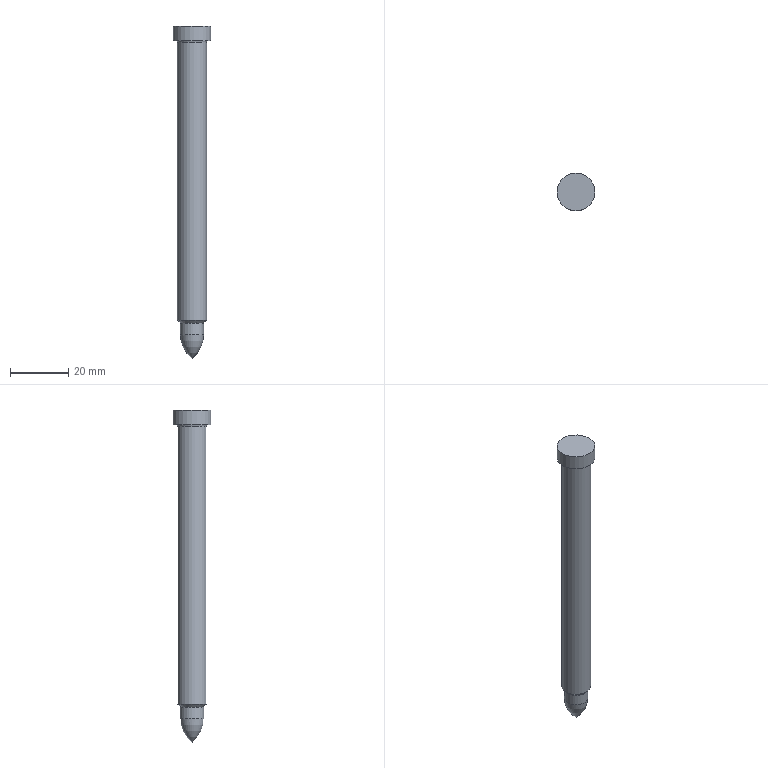Part | NX | features 8 2 | 1 solid | 9 faces | box 13 x 13 x 113.8 mm | volume 8684 mm3 | cylinder 3 | torus 3 | plane 2 | cone 1 | commonest cylinder face diameters 8 x1 10 x1 13 x1
STEP:
#1=CARTESIAN_POINT('',(3285.247,77.328,85.5));
#2=VERTEX_POINT('',#1);
#3=CARTESIAN_POINT('',(3290.247,77.328,85.5));
#4=DIRECTION('',(0.,0.,-1.));
#5=DIRECTION('',(1.,0.,0.));
#6=AXIS2_PLACEMENT_3D('',#3,#4,#5);
#7=CIRCLE('',#6,5.);
#8=EDGE_CURVE('',#2,#2,#7,.T.);
#9=ORIENTED_EDGE('',*,*,#8,.T.);
#10=EDGE_LOOP('',(#9));
#11=FACE_BOUND('',#10,.T.);
#12=CARTESIAN_POINT('',(3285.247,77.328,-9.8));
#13=VERTEX_POINT('',#12);
#14=CARTESIAN_POINT('',(3290.247,77.328,-9.8));
#15=DIRECTION('',(0.,0.,1.));
#16=DIRECTION('',(-1.,0.,0.));
#17=AXIS2_PLACEMENT_3D('',#14,#15,#16);
#18=CIRCLE('',#17,5.);
#19=EDGE_CURVE('',#13,#13,#18,.T.);
#20=ORIENTED_EDGE('',*,*,#19,.T.);
#21=EDGE_LOOP('',(#20));
#22=FACE_BOUND('',#21,.T.);
#23=CARTESIAN_POINT('',(3290.247,77.328,31.));
#24=DIRECTION('',(0.,0.,-1.));
#25=DIRECTION('',(-1.,0.,0.));
#26=AXIS2_PLACEMENT_3D('',#23,#24,#25);
#27=CYLINDRICAL_SURFACE('',#26,5.);
#28=ADVANCED_FACE('',(#11,#22),#27,.T.);
#29=CARTESIAN_POINT('',(3290.247,77.328,-22.8));
#30=VERTEX_POINT('',#29);
#31=VERTEX_LOOP('',#30);
#32=FACE_BOUND('',#31,.T.);
#33=CARTESIAN_POINT('',(3286.247,77.328,-14.8));
#34=VERTEX_POINT('',#33);
#35=CARTESIAN_POINT('',(3290.247,77.328,-14.8));
#36=DIRECTION('',(0.,0.,1.));
#37=DIRECTION('',(-1.,0.,0.));
#38=AXIS2_PLACEMENT_3D('',#35,#36,#37);
#39=CIRCLE('',#38,4.);
#40=EDGE_CURVE('',#34,#34,#39,.T.);
#41=ORIENTED_EDGE('',*,*,#40,.F.);
#42=EDGE_LOOP('',(#41));
#43=FACE_BOUND('',#42,.T.);
#44=CARTESIAN_POINT('',(3290.247,77.328,-14.8));
#45=DIRECTION('',(0.,0.,-1.));
#46=DIRECTION('',(-1.,0.,0.));
#47=AXIS2_PLACEMENT_3D('',#44,#45,#46);
#48=DEGENERATE_TOROIDAL_SURFACE('',#47,6.,10.,.F.);
#49=ADVANCED_FACE('',(#32,#43),#48,.F.);
#50=CARTESIAN_POINT('',(3286.159,77.328,-10.712));
#51=VERTEX_POINT('',#50);
#52=CARTESIAN_POINT('',(3290.247,77.328,-10.712));
#53=DIRECTION('',(0.,0.,1.));
#54=DIRECTION('',(1.,0.,0.));
#55=AXIS2_PLACEMENT_3D('',#52,#53,#54);
#56=CIRCLE('',#55,4.088);
#57=EDGE_CURVE('',#51,#51,#56,.T.);
#58=ORIENTED_EDGE('',*,*,#57,.F.);
#59=EDGE_LOOP('',(#58));
#60=FACE_BOUND('',#59,.T.);
#61=CARTESIAN_POINT('',(3286.247,77.328,-10.924));
#62=VERTEX_POINT('',#61);
#63=CARTESIAN_POINT('',(3290.247,77.328,-10.924));
#64=DIRECTION('',(0.,0.,-1.));
#65=DIRECTION('',(1.,0.,0.));
#66=AXIS2_PLACEMENT_3D('',#63,#64,#65);
#67=CIRCLE('',#66,4.);
#68=EDGE_CURVE('',#62,#62,#67,.T.);
#69=ORIENTED_EDGE('',*,*,#68,.F.);
#70=EDGE_LOOP('',(#69));
#71=FACE_BOUND('',#70,.T.);
#72=CARTESIAN_POINT('',(3290.247,77.328,-10.924));
#73=DIRECTION('',(0.,0.,-1.));
#74=DIRECTION('',(1.,0.,0.));
#75=AXIS2_PLACEMENT_3D('',#72,#73,#74);
#76=TOROIDAL_SURFACE('',#75,4.3,0.3);
#77=ADVANCED_FACE('',(#60,#71),#76,.F.);
#78=ORIENTED_EDGE('',*,*,#40,.T.);
#79=EDGE_LOOP('',(#78));
#80=FACE_BOUND('',#79,.T.);
#81=ORIENTED_EDGE('',*,*,#68,.T.);
#82=EDGE_LOOP('',(#81));
#83=FACE_BOUND('',#82,.T.);
#84=CARTESIAN_POINT('',(3290.247,77.328,-12.8));
#85=DIRECTION('',(0.,0.,-1.));
#86=DIRECTION('',(-1.,0.,0.));
#87=AXIS2_PLACEMENT_3D('',#84,#85,#86);
#88=CYLINDRICAL_SURFACE('',#87,4.);
#89=ADVANCED_FACE('',(#80,#83),#88,.T.);
#90=ORIENTED_EDGE('',*,*,#19,.F.);
#91=EDGE_LOOP('',(#90));
#92=FACE_BOUND('',#91,.T.);
#93=ORIENTED_EDGE('',*,*,#57,.T.);
#94=EDGE_LOOP('',(#93));
#95=FACE_BOUND('',#94,.T.);
#96=CARTESIAN_POINT('',(3290.247,77.328,-10.3));
#97=DIRECTION('',(0.,0.,1.));
#98=DIRECTION('',(-1.,0.,0.));
#99=AXIS2_PLACEMENT_3D('',#96,#97,#98);
#100=CONICAL_SURFACE('',#99,4.5,0.7854);
#101=ADVANCED_FACE('',(#92,#95),#100,.T.);
#102=ORIENTED_EDGE('',*,*,#8,.F.);
#103=EDGE_LOOP('',(#102));
#104=FACE_BOUND('',#103,.T.);
#105=CARTESIAN_POINT('',(3284.747,77.328,86.));
#106=VERTEX_POINT('',#105);
#107=CARTESIAN_POINT('',(3290.247,77.328,86.));
#108=DIRECTION('',(0.,0.,1.));
#109=DIRECTION('',(1.,0.,0.));
#110=AXIS2_PLACEMENT_3D('',#107,#108,#109);
#111=CIRCLE('',#110,5.5);
#112=EDGE_CURVE('',#106,#106,#111,.T.);
#113=ORIENTED_EDGE('',*,*,#112,.F.);
#114=EDGE_LOOP('',(#113));
#115=FACE_BOUND('',#114,.T.);
#116=CARTESIAN_POINT('',(3290.247,77.328,85.5));
#117=DIRECTION('',(0.,0.,1.));
#118=DIRECTION('',(1.,0.,0.));
#119=AXIS2_PLACEMENT_3D('',#116,#117,#118);
#120=TOROIDAL_SURFACE('',#119,5.5,0.5);
#121=ADVANCED_FACE('',(#104,#115),#120,.F.);
#122=CARTESIAN_POINT('',(3283.747,77.328,86.));
#123=VERTEX_POINT('',#122);
#124=CARTESIAN_POINT('',(3290.247,77.328,86.));
#125=DIRECTION('',(0.,0.,1.));
#126=DIRECTION('',(-1.,0.,0.));
#127=AXIS2_PLACEMENT_3D('',#124,#125,#126);
#128=CIRCLE('',#127,6.5);
#129=EDGE_CURVE('',#123,#123,#128,.T.);
#130=ORIENTED_EDGE('',*,*,#129,.F.);
#131=EDGE_LOOP('',(#130));
#132=FACE_BOUND('',#131,.T.);
#133=ORIENTED_EDGE('',*,*,#112,.T.);
#134=EDGE_LOOP('',(#133));
#135=FACE_BOUND('',#134,.T.);
#136=CARTESIAN_POINT('',(3290.247,77.328,86.));
#137=DIRECTION('',(0.,0.,-1.));
#138=DIRECTION('',(-1.,0.,0.));
#139=AXIS2_PLACEMENT_3D('',#136,#137,#138);
#140=PLANE('',#139);
#141=ADVANCED_FACE('',(#132,#135),#140,.T.);
#142=CARTESIAN_POINT('',(3283.747,77.328,91.));
#143=VERTEX_POINT('',#142);
#144=CARTESIAN_POINT('',(3290.247,77.328,91.));
#145=DIRECTION('',(0.,0.,-1.));
#146=DIRECTION('',(-1.,0.,0.));
#147=AXIS2_PLACEMENT_3D('',#144,#145,#146);
#148=CIRCLE('',#147,6.5);
#149=EDGE_CURVE('',#143,#143,#148,.T.);
#150=ORIENTED_EDGE('',*,*,#149,.T.);
#151=EDGE_LOOP('',(#150));
#152=FACE_BOUND('',#151,.T.);
#153=ORIENTED_EDGE('',*,*,#129,.T.);
#154=EDGE_LOOP('',(#153));
#155=FACE_BOUND('',#154,.T.);
#156=CARTESIAN_POINT('',(3290.247,77.328,88.5));
#157=DIRECTION('',(0.,0.,-1.));
#158=DIRECTION('',(-1.,0.,0.));
#159=AXIS2_PLACEMENT_3D('',#156,#157,#158);
#160=CYLINDRICAL_SURFACE('',#159,6.5);
#161=ADVANCED_FACE('',(#152,#155),#160,.T.);
#162=ORIENTED_EDGE('',*,*,#149,.F.);
#163=EDGE_LOOP('',(#162));
#164=FACE_BOUND('',#163,.T.);
#165=CARTESIAN_POINT('',(3290.247,77.328,91.));
#166=DIRECTION('',(0.,0.,1.));
#167=DIRECTION('',(1.,0.,0.));
#168=AXIS2_PLACEMENT_3D('',#165,#166,#167);
#169=PLANE('',#168);
#170=ADVANCED_FACE('',(#164),#169,.T.);
#171=CLOSED_SHELL('',(#28,#49,#77,#89,#101,#121,#141,#161,#170));
#172=MANIFOLD_SOLID_BREP('',#171);
#173=(LENGTH_UNIT()NAMED_UNIT(*)SI_UNIT(.MILLI.,.METRE.));
#174=UNCERTAINTY_MEASURE_WITH_UNIT(LENGTH_MEASURE(0.00001),#173,'','');
#175=(NAMED_UNIT(*)PLANE_ANGLE_UNIT()SI_UNIT($,.RADIAN.));
#176=(NAMED_UNIT(*)SI_UNIT($,.STERADIAN.)SOLID_ANGLE_UNIT());
#177=(GEOMETRIC_REPRESENTATION_CONTEXT(3)GLOBAL_UNCERTAINTY_ASSIGNED_CONTEXT((#174))GLOBAL_UNIT_ASSIGNED_CONTEXT((#173,#175,#176))REPRESENTATION_CONTEXT('',''));
#178=ADVANCED_BREP_SHAPE_REPRESENTATION('',(#172),#177);